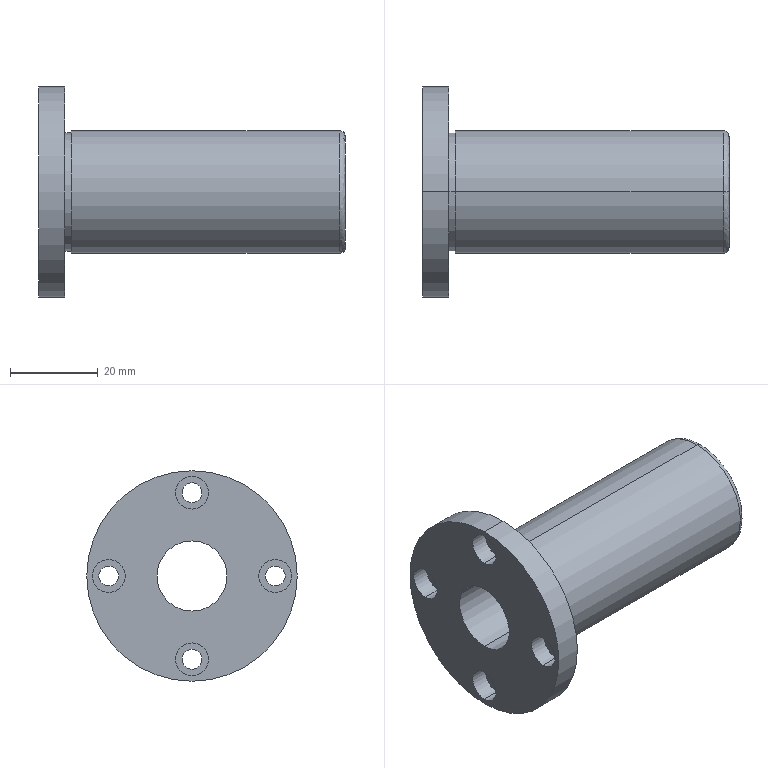Part | STEP file | LHFRW16 | 1 solid | 34 faces | box 70 x 48 x 48 mm | volume 35245 mm3 | cylinder 24 | plane 7 | spline 3 | commonest cylinder face diameters 4.5 x8 7.5 x8 16 x2 27 x2 28 x2 48 x2